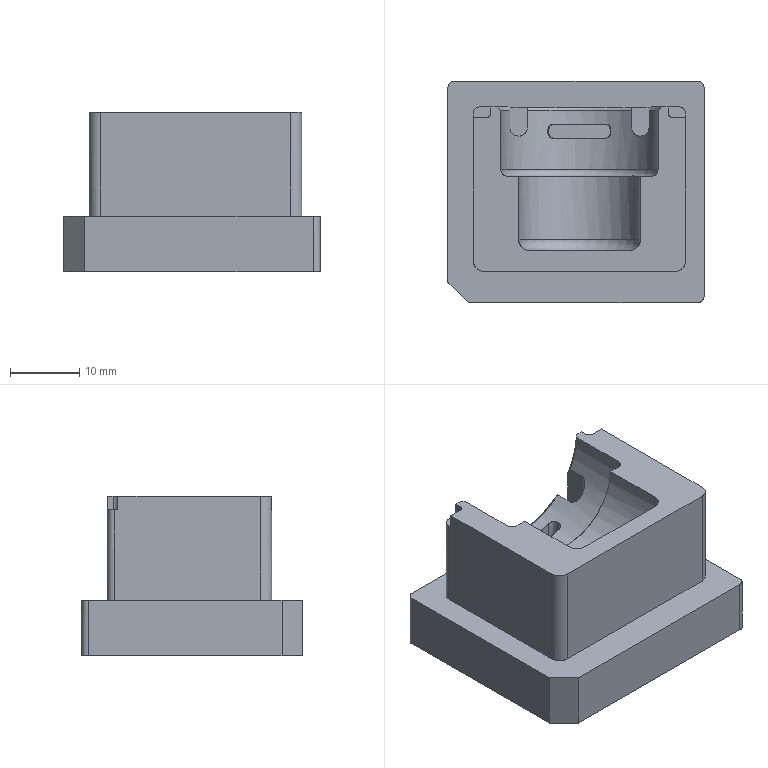NC program | PowerMill | posted with a generic post | part box 37 x 32 x 23 mm
Lines 6224 to 7194 of 159067:
N6321 M6
N6322 S18000 M03
N6323 G00 G90 X0.0 Y0.0
N6324 G43 Z9.8 H15
N6325
N6326 G05 P10000 R4
N6327 X1.8515 Y-13.7996
N6328 Z0.7126
N6329 G01 Z-0.4874 F3000.0
N6330 X1.8602 Y-13.7824 F5000.0
N6331 G03 X1.7827 Y-13.55 I-0.155 J0.0775
N6332 G01 X0.4221 Y-12.8697
N6333 X-13.2972 Y-12.8694
N6334 X-13.7193 Y-12.8327
N6335 X-14.3453 Y-12.664
N6336 X-14.9857 Y-12.3123
N6337 X-15.4079 Y-11.9482
N6338 X-15.8232 Y-11.3976
N6339 X-16.0268 Y-10.9755
N6340 X-16.153 Y-10.5533
N6341 X-16.2131 Y-10.1312
N6342 X-16.2285 Y-9.7091
N6343 Y10.5533
N6344 X-16.2007 Y10.9755
N6345 X-16.0381 Y11.3976
N6346 X-15.83 Y11.6667
N6347 X-15.649 Y11.8197
N6348 X-15.4079 Y11.9557
N6349 X-14.9857 Y12.0648
N6350 X-13.8361 Y12.0701
N6351 G03 X-13.6868 Y12.2419 I-0.0021 J0.1526
N6352 G01 X-13.6241 Y12.664
N6353 X-13.4055 Y13.0861
N6354 X-13.2972 Y13.2114
N6355 X-12.8751 Y13.5055
N6356 X-12.4529 Y13.6177
N6357 X-11.1865 Y13.614
N6358 X-10.7959 Y13.5083
N6359 X-10.3423 Y13.1863
N6360 X-9.8227 Y12.664
N6361 X-9.5656 Y12.2419
N6362 X-9.498 Y12.0011
N6363 X-9.4767 Y11.8197
N6364 X-9.4748 Y3.7248
N6365 G03 X-9.325 Y3.5748 I0.15 J0.0
N6366 G01 X-8.2316 Y3.5737
N6367 X-7.8095 Y3.4916
N6368 X-7.5702 Y3.3771
N6369 X-7.3873 Y3.2447
N6370 X-7.1326 Y2.9549
N6371 X-6.9652 Y2.5935
N6372 X-6.9088 Y2.1107
N6373 Y-6.8878
N6374 X-6.8854 Y-6.9746
N6375 X-6.8807 Y-6.985
N6376 X-6.8154 Y-7.071
N6377 X-6.7168 Y-7.115
N6378 X-6.5431 Y-7.13
N6379 X7.6059
N6380 X7.7172 Y-7.1215
N6381 X7.8143 Y-7.0718
N6382 X7.8801 Y-6.9849
N6383 X7.8902 Y-6.9412
N6384 X7.9046 Y-6.7541
N6385 Y2.1107
N6386 X7.9446 Y2.5328
N6387 X8.1284 Y2.9549
N6388 X8.2316 Y3.092
N6389 X8.5661 Y3.3771
N6390 X8.6537 Y3.4257
N6391 X9.0759 Y3.5548
N6392 X10.3225 Y3.5724
N6393 G03 X10.4704 Y3.7224 I-0.0021 J0.15
N6394 G01 X10.4726 Y11.8197
N6395 X10.5615 Y12.2419
N6396 X10.7644 Y12.5986
N6397 X11.2381 Y13.0861
N6398 X11.6087 Y13.4095
N6399 X11.7917 Y13.5083
N6400 X12.0308 Y13.5852
N6401 X12.4529 Y13.6244
N6402 X13.2972
N6403 X13.7193 Y13.5627
N6404 X13.8649 Y13.5083
N6405 X14.1415 Y13.3453
N6406 X14.4013 Y13.0861
N6407 X14.5636 Y12.8131
N6408 X14.62 Y12.664
N6409 X14.6827 Y12.2419
N6410 G03 X14.8326 Y12.0711 I0.1512 J-0.0185
N6411 G01 X15.83 Y12.0707
N6412 X16.2521 Y12.0118
N6413 X16.6448 Y11.8197
N6414 X17.034 Y11.3976
N6415 X17.0964 Y11.279
N6416 X17.1966 Y10.9755
N6417 X17.2244 Y10.5533
N6418 Y-9.7091
N6419 X17.2089 Y-10.1312
N6420 X17.149 Y-10.5533
N6421 X17.0228 Y-10.9755
N6422 X16.8192 Y-11.3976
N6423 X16.6743 Y-11.6176
N6424 X16.2521 Y-12.0926
N6425 X15.83 Y-12.4168
N6426 X15.3412 Y-12.664
N6427 X14.9857 Y-12.7782
N6428 X14.5636 Y-12.8473
N6429 X14.1415 Y-12.8699
N6430 X0.4221 Y-12.8697
N6431 X1.8515 Y-13.7996 Z-0.6348
N6432 X1.8602 Y-13.7824
N6433 G03 X1.7827 Y-13.55 I-0.155 J0.0775
N6434 G01 X0.4221 Y-12.8697
N6435 X-13.2972 Y-12.8694
N6436 X-13.7193 Y-12.8327
N6437 X-14.3453 Y-12.664
N6438 X-14.9857 Y-12.3123
N6439 X-15.4079 Y-11.9482
N6440 X-15.8232 Y-11.3976
N6441 X-16.0268 Y-10.9755
N6442 X-16.153 Y-10.5533
N6443 X-16.2131 Y-10.1312
N6444 X-16.2285 Y-9.7091
N6445 Y10.5533
N6446 X-16.2007 Y10.9755
N6447 X-16.0381 Y11.3976
N6448 X-15.83 Y11.6667
N6449 X-15.649 Y11.8197
N6450 X-15.4079 Y11.9557
N6451 X-14.9857 Y12.0648
N6452 X-13.8361 Y12.0701
N6453 G03 X-13.6868 Y12.2419 I-0.0022 J0.1527
N6454 G01 X-13.6241 Y12.664
N6455 X-13.4055 Y13.0861
N6456 X-13.2972 Y13.2114
N6457 X-12.8751 Y13.5055
N6458 X-12.4529 Y13.6177
N6459 X-11.1865 Y13.6159
N6460 X-10.7861 Y13.5083
N6461 X-10.3423 Y13.1963
N6462 X-9.8126 Y12.664
N6463 X-9.5556 Y12.2419
N6464 X-9.498 Y12.05
N6465 X-9.4667 Y11.8197
N6466 X-9.4645 Y3.7246
N6467 G03 X-9.3068 Y3.5747 I0.1501 J0.0
N6468 G01 X-9.0376 Y3.5745
N6469 X-8.2316 Y3.574
N6470 X-7.8095 Y3.4963
N6471 X-7.5576 Y3.3771
N6472 X-7.3873 Y3.2551
N6473 X-7.1199 Y2.9549
N6474 X-6.936 Y2.5328
N6475 X-6.8961 Y2.1107
N6476 X-6.8958 Y-6.932
N6477 G03 X-6.7106 Y-7.1136 I0.2343 J0.0537
N6478 G01 X-6.5431 Y-7.1298
N6479 X7.6086 Y-7.1297
N6480 X7.6878 Y-7.1228
N6481 G03 X7.8915 Y-6.9002 I-0.038 J0.2394
N6482 G01 X7.892 Y2.1107
N6483 X7.9319 Y2.5328
N6484 X8.1158 Y2.9549
N6485 X8.2316 Y3.1061
N6486 X8.5535 Y3.3771
N6487 X8.6537 Y3.4322
N6488 X9.0759 Y3.5614
N6489 X10.312 Y3.5731
N6490 G03 X10.4606 Y3.7231 I-0.0014 J0.15
N6491 G01 X10.4625 Y11.8197
N6492 X10.5514 Y12.2419
N6493 X10.7644 Y12.6108
N6494 X11.2283 Y13.0861
N6495 X11.6087 Y13.4166
N6496 X11.7819 Y13.5083
N6497 X12.0308 Y13.5905
N6498 X12.4529 Y13.6244
N6499 X13.2972
N6500 X13.7193 Y13.5627
N6501 X13.8649 Y13.5083
N6502 X14.1415 Y13.3454
N6503 X14.4013 Y13.0861
N6504 X14.5636 Y12.8131
N6505 X14.62 Y12.664
N6506 X14.6827 Y12.2419
N6507 G03 X14.8326 Y12.0711 I0.1512 J-0.0185
N6508 G01 X15.83 Y12.0708
N6509 X16.2521 Y12.0118
N6510 X16.6448 Y11.8197
N6511 X17.034 Y11.3976
N6512 X17.0964 Y11.279
N6513 X17.1966 Y10.9755
N6514 X17.2244 Y10.5533
N6515 Y-9.7091
N6516 X17.2089 Y-10.1312
N6517 X17.149 Y-10.5533
N6518 X17.0228 Y-10.9755
N6519 X16.8192 Y-11.3976
N6520 X16.6743 Y-11.6176
N6521 X16.2521 Y-12.0926
N6522 X15.83 Y-12.4168
N6523 X15.3412 Y-12.664
N6524 X14.9857 Y-12.7782
N6525 X14.5636 Y-12.8473
N6526 X14.1415 Y-12.8699
N6527 X0.4221 Y-12.8697
N6528 X1.8515 Y-13.7996 Z-0.7821
N6529 X1.8602 Y-13.7824
N6530 G03 X1.7827 Y-13.55 I-0.155 J0.0775
N6531 G01 X0.4221 Y-12.8697
N6532 X-13.2972 Y-12.8694
N6533 X-13.7193 Y-12.8327
N6534 X-14.3453 Y-12.664
N6535 X-14.9857 Y-12.3123
N6536 X-15.4079 Y-11.9482
N6537 X-15.8232 Y-11.3976
N6538 X-16.0268 Y-10.9755
N6539 X-16.153 Y-10.5533
N6540 X-16.2131 Y-10.1312
N6541 X-16.2285 Y-9.7091
N6542 Y10.5533
N6543 X-16.2007 Y10.9755
N6544 X-16.0381 Y11.3976
N6545 X-15.83 Y11.6667
N6546 X-15.649 Y11.8197
N6547 X-15.4079 Y11.9557
N6548 X-14.9857 Y12.0648
N6549 X-13.8361 Y12.0701
N6550 G03 X-13.6868 Y12.2312 I-0.0011 J0.1507
N6551 G01 Y12.2419
N6552 X-13.6241 Y12.664
N6553 X-13.4055 Y13.0861
N6554 X-13.2972 Y13.2114
N6555 X-12.8751 Y13.5055
N6556 X-12.4529 Y13.6177
N6557 X-11.1865 Y13.617
N6558 X-10.7644 Y13.5029
N6559 X-10.3423 Y13.2062
N6560 X-9.8026 Y12.664
N6561 X-9.5455 Y12.2419
N6562 X-9.498 Y12.0927
N6563 X-9.4566 Y11.8197
N6564 X-9.4542 Y3.7252
N6565 G03 X-9.3043 Y3.5753 I0.15 J0.0001
N6566 G01 X-8.2316 Y3.5743
N6567 X-7.8095 Y3.501
N6568 X-7.545 Y3.3771
N6569 X-7.3873 Y3.2656
N6570 X-7.1073 Y2.9549
N6571 X-6.9652 Y2.6697
N6572 X-6.9234 Y2.5328
N6573 X-6.8835 Y2.1107
N6574 X-6.8838 Y-6.9302
N6575 G03 X-6.7045 Y-7.1114 I0.2297 J0.048
N6576 G01 X-6.5431 Y-7.1297
N6577 X7.6111 Y-7.1286
N6578 X7.6889 Y-7.119
N6579 X7.7838 Y-7.0767
N6580 X7.8508 Y-6.9972
N6581 X7.8796 Y-6.9246
N6582 X7.8794 Y2.1107
N6583 X7.9193 Y2.5328
N6584 X8.1032 Y2.9549
N6585 X8.2316 Y3.1202
N6586 X8.5408 Y3.3771
N6587 X8.6537 Y3.4387
N6588 X9.0759 Y3.5634
N6589 X10.3015 Y3.5733
N6590 G03 X10.4503 Y3.7233 I-0.0012 J0.15
N6591 G01 X10.4525 Y11.8197
N6592 X10.5413 Y12.2419
N6593 X10.7644 Y12.6229
N6594 X11.2185 Y13.0861
N6595 X11.6087 Y13.4225
N6596 X11.7722 Y13.5083
N6597 X12.0308 Y13.5928
N6598 X12.4529 Y13.6244
N6599 X13.2972
N6600 X13.7193 Y13.5627
N6601 X13.865 Y13.5083
N6602 X14.1415 Y13.3454
N6603 X14.4013 Y13.0861
N6604 X14.5636 Y12.8131
N6605 X14.62 Y12.664
N6606 X14.6827 Y12.2419
N6607 G03 X14.8327 Y12.0711 I0.1513 J-0.0185
N6608 G01 X15.83 Y12.0708
N6609 X16.2521 Y12.0118
N6610 X16.6448 Y11.8197
N6611 X17.034 Y11.3976
N6612 X17.0964 Y11.279
N6613 X17.1966 Y10.9755
N6614 X17.2244 Y10.5533
N6615 Y-9.7091
N6616 X17.2089 Y-10.1312
N6617 X17.149 Y-10.5533
N6618 X17.0228 Y-10.9755
N6619 X16.8192 Y-11.3976
N6620 X16.6743 Y-11.6176
N6621 X16.2521 Y-12.0926
N6622 X15.83 Y-12.4168
N6623 X15.3412 Y-12.664
N6624 X14.9857 Y-12.7782
N6625 X14.5636 Y-12.8473
N6626 X14.1415 Y-12.8699
N6627 X0.4221 Y-12.8697
N6628 X1.8515 Y-13.7996 Z-0.9295
N6629 X1.8602 Y-13.7824
N6630 G03 X1.7827 Y-13.55 I-0.155 J0.0775
N6631 G01 X0.4221 Y-12.8697
N6632 X-13.2972 Y-12.8694
N6633 X-13.7193 Y-12.8327
N6634 X-14.3453 Y-12.664
N6635 X-14.9857 Y-12.3123
N6636 X-15.4079 Y-11.9482
N6637 X-15.8232 Y-11.3976
N6638 X-16.0268 Y-10.9755
N6639 X-16.153 Y-10.5533
N6640 X-16.2131 Y-10.1312
N6641 X-16.2285 Y-9.7091
N6642 Y10.5533
N6643 X-16.2007 Y10.9755
N6644 X-16.0381 Y11.3976
N6645 X-15.83 Y11.6667
N6646 X-15.649 Y11.8197
N6647 X-15.4079 Y11.9557
N6648 X-14.9857 Y12.0648
N6649 X-13.8362 Y12.0701
N6650 G03 X-13.6868 Y12.2419 I-0.0021 J0.1527
N6651 G01 X-13.6242 Y12.664
N6652 X-13.4055 Y13.0861
N6653 X-13.2972 Y13.2114
N6654 X-12.8751 Y13.5055
N6655 X-12.4529 Y13.6177
N6656 X-11.1865 Y13.618
N6657 X-10.7666 Y13.5083
N6658 X-10.3423 Y13.2161
N6659 X-9.7925 Y12.664
N6660 X-9.5354 Y12.2419
N6661 X-9.5056 Y12.1155
N6662 X-9.4819 Y11.9878
N6663 X-9.4465 Y11.8197
N6664 X-9.4439 Y3.7252
N6665 G03 X-9.294 Y3.5752 I0.15 J0.0
N6666 G01 X-8.2316 Y3.5744
N6667 X-7.8095 Y3.5056
N6668 X-7.5323 Y3.3771
N6669 X-7.3873 Y3.2761
N6670 X-7.0946 Y2.9549
N6671 X-6.9652 Y2.7039
N6672 X-6.9108 Y2.5328
N6673 X-6.8708 Y2.1107
N6674 Y-6.8838
N6675 X-6.859 Y-6.9487
N6676 X-6.8369 Y-7.0107
N6677 X-6.7776 Y-7.0739
N6678 X-6.6984 Y-7.1091
N6679 X-6.5431 Y-7.1296
N6680 X7.6132 Y-7.1271
N6681 X7.6703 Y-7.1192
N6682 X7.7259 Y-7.104
N6683 X7.7968 Y-7.0548
N6684 X7.8452 Y-6.9834
N6685 X7.8668 Y-6.9154
N6686 X7.8667 Y2.1107
N6687 X7.9066 Y2.5328
N6688 X8.0905 Y2.9549
N6689 X8.2316 Y3.1343
N6690 X8.5282 Y3.3771
N6691 X8.6537 Y3.4451
N6692 X9.0759 Y3.565
N6693 X10.2912 Y3.5735
N6694 G03 X10.4401 Y3.7234 I-0.0011 J0.15
N6695 G01 X10.4424 Y11.8197
N6696 X10.5311 Y12.2419
N6697 X10.7644 Y12.6351
N6698 X11.2088 Y13.0861
N6699 X11.6087 Y13.4284
N6700 X11.7625 Y13.5083
N6701 X12.0308 Y13.5952
N6702 X12.4529 Y13.6244
N6703 X13.2972
N6704 X13.7193 Y13.5627
N6705 X13.865 Y13.5083
N6706 X14.1415 Y13.3454
N6707 X14.4013 Y13.0861
N6708 X14.5636 Y12.8131
N6709 X14.62 Y12.664
N6710 X14.6827 Y12.2419
N6711 G03 X14.8327 Y12.0711 I0.1513 J-0.0185
N6712 G01 X15.83 Y12.0708
N6713 X16.2521 Y12.0118
N6714 X16.6448 Y11.8197
N6715 X17.034 Y11.3976
N6716 X17.0964 Y11.279
N6717 X17.1966 Y10.9755
N6718 X17.2244 Y10.5533
N6719 Y-9.7091
N6720 X17.2089 Y-10.1312
N6721 X17.149 Y-10.5533
N6722 X17.0228 Y-10.9755
N6723 X16.8192 Y-11.3976
N6724 X16.6743 Y-11.6176
N6725 X16.2521 Y-12.0926
N6726 X15.83 Y-12.4168
N6727 X15.3412 Y-12.664
N6728 X14.9857 Y-12.7782
N6729 X14.5636 Y-12.8474
N6730 X14.1415 Y-12.8699
N6731 X0.4221 Y-12.8697
N6732 X1.8515 Y-13.7996 Z-1.0769
N6733 X1.8602 Y-13.7824
N6734 G03 X1.7827 Y-13.55 I-0.155 J0.0775
N6735 G01 X0.4221 Y-12.8697
N6736 X-13.2972 Y-12.8694
N6737 X-13.7193 Y-12.8327
N6738 X-14.3453 Y-12.664
N6739 X-14.9857 Y-12.3123
N6740 X-15.4079 Y-11.9482
N6741 X-15.8232 Y-11.3976
N6742 X-16.0268 Y-10.9755
N6743 X-16.153 Y-10.5533
N6744 X-16.2131 Y-10.1312
N6745 X-16.2285 Y-9.7091
N6746 Y10.5533
N6747 X-16.2007 Y10.9755
N6748 X-16.0381 Y11.3976
N6749 X-15.83 Y11.6667
N6750 X-15.649 Y11.8197
N6751 X-15.4079 Y11.9558
N6752 X-14.9857 Y12.0648
N6753 X-13.8362 Y12.0701
N6754 G03 X-13.6868 Y12.2419 I-0.0021 J0.1527
N6755 G01 X-13.6242 Y12.664
N6756 X-13.4055 Y13.0861
N6757 X-13.2972 Y13.2114
N6758 X-12.8751 Y13.5055
N6759 X-12.4529 Y13.6177
N6760 X-11.1865 Y13.6189
N6761 X-10.7644 Y13.5121
N6762 X-10.3423 Y13.226
N6763 X-9.7824 Y12.664
N6764 X-9.5253 Y12.2419
N6765 X-9.4364 Y11.8197
N6766 X-9.4335 Y3.7252
N6767 G03 X-9.2837 Y3.5752 I0.15 J0.0
N6768 G01 X-8.2316 Y3.5744
N6769 X-7.8095 Y3.5103
N6770 X-7.5197 Y3.3771
N6771 X-7.3873 Y3.2865
N6772 X-7.082 Y2.9549
N6773 X-6.9652 Y2.7345
N6774 X-6.8981 Y2.5328
N6775 X-6.8582 Y2.1107
N6776 Y-6.8825
N6777 X-6.8462 Y-6.9457
N6778 X-6.8245 Y-7.0062
N6779 X-6.7949 Y-7.043
N6780 X-6.7588 Y-7.0735
N6781 X-6.7274 Y-7.0938
N6782 X-6.6916 Y-7.1045
N6783 X-6.5431 Y-7.1294
N6784 X-5.6685 Y-7.1295
N6785 X7.5067 Y-7.1272
N6786 X7.6208 Y-7.1245
N6787 X7.729 Y-7.0847
N6788 X7.8161 Y-7.0084
N6789 X7.854 Y-6.899
N6790 X7.8541 Y2.1107
N6791 X7.894 Y2.5328
N6792 X8.0779 Y2.9549
N6793 X8.2316 Y3.1485
N6794 X8.5156 Y3.3771
N6795 X8.6537 Y3.4516
N6796 X9.0759 Y3.5664
N6797 X10.2809 Y3.5736
N6798 G03 X10.43 Y3.7236 I-0.0009 J0.15
N6799 G01 X10.4323 Y11.8197
N6800 X10.521 Y12.2419
N6801 X10.7644 Y12.6472
N6802 X11.1865 Y13.0736
N6803 X11.6087 Y13.4344
N6804 X11.7527 Y13.5083
N6805 X12.0308 Y13.5975
N6806 X12.4529 Y13.6244
N6807 X13.2972
N6808 X13.7193 Y13.5628
N6809 X13.865 Y13.5083
N6810 X14.1415 Y13.3454
N6811 X14.4013 Y13.0861
N6812 X14.5636 Y12.8131
N6813 X14.62 Y12.664
N6814 X14.6827 Y12.2419
N6815 G03 X14.8327 Y12.0711 I0.1513 J-0.0185
N6816 G01 X15.83 Y12.0708
N6817 X16.2521 Y12.0118
N6818 X16.6448 Y11.8197
N6819 X17.034 Y11.3976
N6820 X17.0964 Y11.279
N6821 X17.1966 Y10.9755
N6822 X17.2244 Y10.5533
N6823 Y-9.7091
N6824 X17.2089 Y-10.1312
N6825 X17.149 Y-10.5533
N6826 X17.0228 Y-10.9755
N6827 X16.8192 Y-11.3976
N6828 X16.6743 Y-11.6176
N6829 X16.2521 Y-12.0926
N6830 X15.83 Y-12.4168
N6831 X15.3412 Y-12.664
N6832 X14.9857 Y-12.7782
N6833 X14.5636 Y-12.8474
N6834 X14.1415 Y-12.87
N6835 X0.4221 Y-12.8697
N6836 X1.8515 Y-13.7996 Z-1.2243
N6837 X1.8602 Y-13.7824
N6838 G03 X1.7827 Y-13.55 I-0.155 J0.0775
N6839 G01 X0.4221 Y-12.8697
N6840 X-13.2972 Y-12.8694
N6841 X-13.7193 Y-12.8327
N6842 X-14.3453 Y-12.664
N6843 X-14.9857 Y-12.3123
N6844 X-15.4079 Y-11.9482
N6845 X-15.8232 Y-11.3976
N6846 X-16.0268 Y-10.9755
N6847 X-16.153 Y-10.5533
N6848 X-16.2131 Y-10.1312
N6849 X-16.2285 Y-9.7091
N6850 Y10.5533
N6851 X-16.2008 Y10.9755
N6852 X-16.0381 Y11.3976
N6853 X-15.83 Y11.6667
N6854 X-15.649 Y11.8197
N6855 X-15.4079 Y11.9558
N6856 X-14.9857 Y12.0649
N6857 X-13.8362 Y12.0701
N6858 G03 X-13.6868 Y12.2419 I-0.0021 J0.1526
N6859 G01 X-13.6242 Y12.664
N6860 X-13.4055 Y13.0861
N6861 X-13.2972 Y13.2115
N6862 X-12.8751 Y13.5056
N6863 X-12.4529 Y13.6177
N6864 X-11.1865 Y13.6198
N6865 X-10.7644 Y13.5169
N6866 X-10.3423 Y13.2359
N6867 X-9.7723 Y12.664
N6868 X-9.5153 Y12.2419
N6869 X-9.4264 Y11.8197
N6870 X-9.4232 Y3.7245
N6871 X-9.4007 Y3.6456
N6872 X-9.34 Y3.5903
N6873 X-9.3065 Y3.5808
N6874 X-9.2867 Y3.5766
N6875 X-9.2664 Y3.5752
N6876 X-8.3208 Y3.5744
N6877 X-8.2316
N6878 X-7.8095 Y3.515
N6879 X-7.5052 Y3.3771
N6880 X-7.3873 Y3.297
N6881 X-7.068 Y2.9549
N6882 X-6.9652 Y2.7653
N6883 X-6.8833 Y2.5328
N6884 X-6.8456 Y2.1107
N6885 X-6.8419 Y-6.8796
N6886 X-6.8029 Y-6.997
N6887 X-6.7898 Y-7.0264
N6888 X-6.7691 Y-7.0512
N6889 X-6.7554 Y-7.0645
N6890 X-6.7401 Y-7.076
N6891 X-6.7239 Y-7.0866
N6892 X-6.689 Y-7.0986
N6893 X-6.5431 Y-7.1293
N6894 X-4.8657 Y-7.1294
N6895 X7.4658 Y-7.1272
N6896 X7.5983 Y-7.1226
N6897 X7.6337 Y-7.1172
N6898 X7.6667 Y-7.1035
N6899 X7.7258 Y-7.0716
N6900 X7.7782 Y-7.0297
N6901 X7.8048 Y-6.9831
N6902 X7.8409 Y-6.8809
N6903 X7.8414 Y2.1107
N6904 X7.8796 Y2.5328
N6905 X8.0634 Y2.9549
N6906 X8.2316 Y3.1641
N6907 X8.5014 Y3.3771
N6908 X8.6537 Y3.4581
N6909 X9.0759 Y3.568
N6910 X10.2705 Y3.5738
N6911 G03 X10.4198 Y3.7237 I-0.0007 J0.15
N6912 G01 X10.4222 Y11.8197
N6913 X10.5109 Y12.2419
N6914 X10.7644 Y12.6594
N6915 X11.1865 Y13.0834
N6916 X11.6087 Y13.4403
N6917 X11.743 Y13.5083
N6918 X12.0308 Y13.5998
N6919 X12.4529 Y13.6244
N6920 X13.2972
N6921 X13.7193 Y13.5628
N6922 X13.865 Y13.5083
N6923 X14.1415 Y13.3454
N6924 X14.4014 Y13.0861
N6925 X14.5636 Y12.8131
N6926 X14.62 Y12.664
N6927 X14.6827 Y12.2419
N6928 G03 X14.8327 Y12.0711 I0.1513 J-0.0185
N6929 G01 X15.83 Y12.0708
N6930 X16.2521 Y12.0118
N6931 X16.6448 Y11.8197
N6932 X17.034 Y11.3976
N6933 X17.0964 Y11.279
N6934 X17.1966 Y10.9755
N6935 X17.2244 Y10.5533
N6936 Y-9.7091
N6937 X17.2089 Y-10.1312
N6938 X17.149 Y-10.5533
N6939 X17.0228 Y-10.9755
N6940 X16.8192 Y-11.3976
N6941 X16.6743 Y-11.6176
N6942 X16.2521 Y-12.0926
N6943 X15.83 Y-12.4168
N6944 X15.3412 Y-12.664
N6945 X14.9857 Y-12.7782
N6946 X14.5636 Y-12.8474
N6947 X14.1415 Y-12.87
N6948 X0.4221 Y-12.8697
N6949 X1.8515 Y-13.7996 Z-1.3717
N6950 X1.8602 Y-13.7824
N6951 G03 X1.7827 Y-13.55 I-0.155 J0.0775
N6952 G01 X0.4221 Y-12.8697
N6953 X-13.2972 Y-12.8694
N6954 X-13.7193 Y-12.8327
N6955 X-14.3453 Y-12.664
N6956 X-14.9857 Y-12.3123
N6957 X-15.4079 Y-11.9482
N6958 X-15.8232 Y-11.3976
N6959 X-16.0268 Y-10.9755
N6960 X-16.153 Y-10.5533
N6961 X-16.2131 Y-10.1312
N6962 X-16.2285 Y-9.7091
N6963 Y10.5533
N6964 X-16.2008 Y10.9755
N6965 X-16.0382 Y11.3976
N6966 X-15.83 Y11.6667
N6967 X-15.6491 Y11.8197
N6968 X-15.4079 Y11.9558
N6969 X-14.9857 Y12.0649
N6970 X-13.8362 Y12.0701
N6971 G03 X-13.6868 Y12.2419 I-0.0021 J0.1526
N6972 G01 X-13.6242 Y12.664
N6973 X-13.4056 Y13.0861
N6974 X-13.2972 Y13.2115
N6975 X-12.8751 Y13.5056
N6976 X-12.4529 Y13.6177
N6977 X-11.1865 Y13.6208
N6978 X-10.7644 Y13.5218
N6979 X-10.3423 Y13.2476
N6980 X-9.7593 Y12.664
N6981 X-9.5035 Y12.2419
N6982 X-9.4141 Y11.8197
N6983 X-9.4129 Y3.7248
N6984 G03 X-9.254 Y3.5751 I0.1499 J0.0
N6985 G01 X-8.5013 Y3.5745
N6986 X-8.2316 Y3.5744
N6987 X-7.8095 Y3.5199
N6988 X-7.4839 Y3.3771
N6989 X-7.3873 Y3.3128
N6990 X-7.0457 Y2.9549
N6991 X-6.9652 Y2.8121
N6992 X-6.8616 Y2.5328
N6993 X-6.8256 Y2.1107
N6994 X-6.8281 Y-6.7541
N6995 X-6.8143 Y-6.9106
N6996 X-6.7786 Y-6.9999
N6997 X-6.7147 Y-7.0717
N6998 X-6.668 Y-7.0936
N6999 X-6.5431 Y-7.1277
N7000 X-0.6247 Y-7.1287
N7001 X7.4658 Y-7.1273
N7002 X7.578 Y-7.1196
N7003 X7.6861 Y-7.0888
N7004 X7.7597 Y-7.0231
N7005 X7.8019 Y-6.934
N7006 X7.824 Y-6.7541
N7007 Y1.2664
N7008 X7.8204 Y2.1107
N7009 X7.8575 Y2.5328
N7010 X8.0421 Y2.9549
N7011 X8.2316 Y3.1855
N7012 X8.4792 Y3.3771
N7013 X8.6537 Y3.466
N7014 X9.0759 Y3.5698
N7015 X10.2603 Y3.574
N7016 G03 X10.4098 Y3.724 I-0.0005 J0.15
N7017 G01 X10.409 Y11.8197
N7018 X10.4997 Y12.2419
N7019 X10.7549 Y12.664
N7020 X11.1865 Y13.0959
N7021 X11.6087 Y13.4476
N7022 X11.7288 Y13.5083
N7023 X12.0308 Y13.6021
N7024 X12.0888 Y13.6031
N7025 X12.4529 Y13.6244
N7026 X13.2943
N7027 X13.2972
N7028 X13.7193 Y13.5628
N7029 X13.865 Y13.5083
N7030 X14.1415 Y13.3454
N7031 X14.4014 Y13.0861
N7032 X14.5636 Y12.8131
N7033 X14.62 Y12.664
N7034 X14.6827 Y12.2419
N7035 G03 X14.8327 Y12.0711 I0.1513 J-0.0185
N7036 G01 X15.83 Y12.0708
N7037 X16.2521 Y12.0118
N7038 X16.6448 Y11.8197
N7039 X17.034 Y11.3976
N7040 X17.0964 Y11.279
N7041 X17.1966 Y10.9755
N7042 X17.2244 Y10.5533
N7043 Y-9.7091
N7044 X17.2089 Y-10.1312
N7045 X17.149 Y-10.5533
N7046 X17.0228 Y-10.9755
N7047 X16.8192 Y-11.3976
N7048 X16.6743 Y-11.6176
N7049 X16.2521 Y-12.0926
N7050 X15.83 Y-12.4168
N7051 X15.3412 Y-12.664
N7052 X14.9857 Y-12.7782
N7053 X14.5636 Y-12.8474
N7054 X14.1415 Y-12.87
N7055 X0.4221 Y-12.8697
N7056 X1.8515 Y-13.7996 Z-1.5191
N7057 X1.8602 Y-13.7824
N7058 G03 X1.7827 Y-13.55 I-0.155 J0.0775
N7059 G01 X0.4221 Y-12.8697
N7060 X-13.2972 Y-12.8694
N7061 X-13.7193 Y-12.8327
N7062 X-14.3453 Y-12.664
N7063 X-14.9857 Y-12.3123
N7064 X-15.4079 Y-11.9482
N7065 X-15.8232 Y-11.3976
N7066 X-16.0269 Y-10.9755
N7067 X-16.153 Y-10.5533
N7068 X-16.2131 Y-10.1312
N7069 X-16.2285 Y-9.7091
N7070 Y10.5533
N7071 X-16.2008 Y10.9755
N7072 X-16.0382 Y11.3976
N7073 X-15.83 Y11.6667
N7074 X-15.6491 Y11.8197
N7075 X-15.4079 Y11.9558
N7076 X-14.9857 Y12.0649
N7077 X-13.8362 Y12.0701
N7078 G03 X-13.6868 Y12.2419 I-0.0021 J0.1526
N7079 G01 X-13.6242 Y12.664
N7080 X-13.4056 Y13.0861
N7081 X-13.2972 Y13.2115
N7082 X-12.8751 Y13.5056
N7083 X-12.4529 Y13.6177
N7084 X-11.1865 Y13.622
N7085 X-10.7644 Y13.5292
N7086 X-10.3423 Y13.2664
N7087 X-9.7386 Y12.664
N7088 X-9.498 Y12.2823
N7089 X-9.3926 Y11.8197
N7090 X-9.3924 Y3.7249
N7091 G03 X-9.249 Y3.5751 I0.15 J0.0
N7092 G01 X-8.7766 Y3.5747
N7093 X-8.2316 Y3.5744
N7094 X-7.8095 Y3.5269
N7095 X-7.5569 Y3.409
N7096 X-7.484 Y3.377
N7097 X-7.4738 Y3.3702
N7098 X-7.3873 Y3.3299
N7099 X-7.022 Y2.9549
N7100 X-6.8374 Y2.5328
N7101 X-6.7983 Y2.1107
N7102 Y-6.8732
N7103 X-6.7803 Y-6.9459
N7104 X-6.7511 Y-7.0149
N7105 X-6.7094 Y-7.0583
N7106 X-6.6591 Y-7.0913
N7107 X-6.6325 Y-7.1028
N7108 X-6.6043 Y-7.1089
N7109 X-6.5971 Y-7.1097
N7110 X-6.1709 Y-7.1279
N7111 X-0.6247 Y-7.1287
N7112 X7.4238 Y-7.1273
N7113 X7.5832 Y-7.116
N7114 X7.6906 Y-7.0703
N7115 X7.7635 Y-6.9791
N7116 X7.7922 Y-6.891
N7117 X7.7941 Y2.1107
N7118 X7.834 Y2.5328
N7119 X8.0176 Y2.9549
N7120 X8.2316 Y3.2089
N7121 X8.4553 Y3.3771
N7122 X8.6537 Y3.4763
N7123 X9.0759 Y3.5717
N7124 X10.2376 Y3.5742
N7125 G03 X10.3873 Y3.7242 I-0.0003 J0.15
N7126 G01 Y11.8197
N7127 X10.4766 Y12.2419
N7128 X10.7333 Y12.664
N7129 X11.1865 Y13.1156
N7130 X11.6087 Y13.4587
N7131 X11.8182 Y13.5363
N7132 X12.0308 Y13.6049
N7133 X12.2421 Y13.6101
N7134 X12.4529 Y13.6243
N7135 X13.2907
N7136 X13.2972 Y13.6244
N7137 X13.7193 Y13.5628
N7138 X13.865 Y13.5083
N7139 X14.1415 Y13.3454
N7140 X14.4014 Y13.0861
N7141 X14.5636 Y12.8131
N7142 X14.6201 Y12.664
N7143 X14.6827 Y12.2419
N7144 G03 X14.8327 Y12.0711 I0.1513 J-0.0185
N7145 G01 X15.83 Y12.0708
N7146 X16.2521 Y12.0118
N7147 X16.6448 Y11.8197
N7148 X17.034 Y11.3976
N7149 X17.0964 Y11.2791
N7150 X17.1966 Y10.9755
N7151 X17.2244 Y10.5533
N7152 Y-9.7091
N7153 X17.2089 Y-10.1312
N7154 X17.149 Y-10.5533
N7155 X17.0228 Y-10.9755
N7156 X16.8192 Y-11.3976
N7157 X16.6743 Y-11.6176
N7158 X16.2521 Y-12.0926
N7159 X15.83 Y-12.4168
N7160 X15.3412 Y-12.664
N7161 X14.9857 Y-12.7782
N7162 X14.5636 Y-12.8474
N7163 X14.1415 Y-12.87
N7164 X0.4221 Y-12.8697
N7165 X1.8515 Y-13.7996 Z-1.6665
N7166 X1.8602 Y-13.7824
N7167 G03 X1.7827 Y-13.55 I-0.155 J0.0775
N7168 G01 X0.4221 Y-12.8697
N7169 X-13.2972 Y-12.8694
N7170 X-13.7193 Y-12.8327
N7171 X-14.3453 Y-12.664
N7172 X-14.9857 Y-12.3123
N7173 X-15.4079 Y-11.9482
N7174 X-15.8232 Y-11.3976
N7175 X-16.0269 Y-10.9755
N7176 X-16.153 Y-10.5533
N7177 X-16.2131 Y-10.1312
N7178 X-16.2285 Y-9.7091
N7179 Y10.5533
N7180 X-16.2008 Y10.9755
N7181 X-16.0382 Y11.3976
N7182 X-15.83 Y11.6668
N7183 X-15.6491 Y11.8197
N7184 X-15.4079 Y11.9558
N7185 X-14.9857 Y12.0649
N7186 X-13.8362 Y12.0701
N7187 G03 X-13.6868 Y12.2419 I-0.0021 J0.1526
N7188 G01 X-13.6242 Y12.664
N7189 X-13.4056 Y13.0861
N7190 X-13.2972 Y13.2115
N7191 X-12.8751 Y13.5056
N7192 X-12.4529 Y13.6178
N7193 X-11.1865 Y13.6232
N7194 X-10.7644 Y13.537
N7195 X-10.3423 Y13.2852
N7196 X-9.7147 Y12.664
N7197 X-9.4576 Y12.2419
N7198 X-9.3687 Y11.8197
N7199 X-9.3678 Y3.7247
N7200 G03 X-9.2275 Y3.575 I0.15 J0.0
N7201 G01 X-8.7766 Y3.5746
N7202 X-8.466 Y3.5745
N7203 X-8.2316 Y3.5744
N7204 X-7.8095 Y3.5339
N7205 X-7.4293 Y3.3771
N7206 X-6.9921 Y2.9549
N7207 X-6.8083 Y2.5328
N7208 X-6.7684 Y2.1107
N7209 X-6.7682 Y-6.9075
N7210 X-6.7423 Y-6.9963
N7211 X-6.6787 Y-7.0633
N7212 X-6.6257 Y-7.0928
N7213 X-6.5941 Y-7.1059
N7214 X-6.5604 Y-7.1113
N7215 X-6.1709 Y-7.1279
N7216 X-0.6247 Y-7.1288
N7217 X7.413 Y-7.1274
N7218 X7.5786 Y-7.111
N7219 X7.6565 Y-7.0824
N7220 X7.7153 Y-7.0238
N7221 X7.7492 Y-6.9639
N7222 X7.7648 Y-6.8968
N7223 X7.7643 Y2.1107
N7224 X7.8042 Y2.5328
N7225 X7.9881 Y2.9549
N7226 X8.2316 Y3.2342
N7227 X8.4256 Y3.3771
N7228 X8.6537 Y3.4865
N7229 X9.0759 Y3.5732
N7230 X10.2133 Y3.5744
N7231 G03 X10.3632 Y3.7243 I-0.0001 J0.15
N7232 G01 X10.3635 Y11.8197
N7233 X10.4535 Y12.2419
N7234 X10.7096 Y12.664
N7235 X11.1865 Y13.1384
N7236 X11.6087 Y13.4698
N7237 X12.0308 Y13.6083
N7238 X12.2421 Y13.6115
N7239 X12.4529 Y13.6243
N7240 X13.2853
N7241 X13.2972 Y13.6244
N7242 X13.7193 Y13.5628
N7243 X13.865 Y13.5083
N7244 X14.1415 Y13.3454
N7245 X14.4014 Y13.0861
N7246 X14.5636 Y12.8131
N7247 X14.6201 Y12.664
N7248 X14.6828 Y12.2419
N7249 G03 X14.8327 Y12.0711 I0.1512 J-0.0185
N7250 G01 X15.83 Y12.0708
N7251 X16.2521 Y12.0118
N7252 X16.6448 Y11.8197
N7253 X17.034 Y11.3976
N7254 X17.0964 Y11.2791
N7255 X17.1966 Y10.9755
N7256 X17.2244 Y10.5533
N7257 Y-9.7091
N7258 X17.2089 Y-10.1312
N7259 X17.149 Y-10.5533
N7260 X17.0228 Y-10.9755
N7261 X16.8192 Y-11.3976
N7262 X16.6743 Y-11.6176
N7263 X16.2521 Y-12.0926
N7264 X15.83 Y-12.4168
N7265 X15.3412 Y-12.664
N7266 X14.9857 Y-12.7782
N7267 X14.5636 Y-12.8474
N7268 X14.1415 Y-12.87
N7269 X0.4221 Y-12.8697
N7270 X1.8515 Y-13.7997 Z-1.8138
N7271 X1.8602 Y-13.7824
N7272 G03 X1.7827 Y-13.55 I-0.155 J0.0775
N7273 G01 X0.4221 Y-12.8697
N7274 X-13.2972 Y-12.8694
N7275 X-13.7193 Y-12.8327
N7276 X-14.3453 Y-12.664
N7277 X-14.9857 Y-12.3123
N7278 X-15.4079 Y-11.9482
N7279 X-15.8232 Y-11.3976
N7280 X-16.0269 Y-10.9755
N7281 X-16.153 Y-10.5533
N7282 X-16.2131 Y-10.1312
N7283 X-16.2285 Y-9.7091
N7284 Y10.5533
N7285 X-16.2008 Y10.9755
N7286 X-16.0382 Y11.3976
N7287 X-15.83 Y11.6668
N7288 X-15.6491 Y11.8197
N7289 X-15.4079 Y11.9558
N7290 X-14.9857 Y12.0649
N7291 X-13.8362 Y12.0701